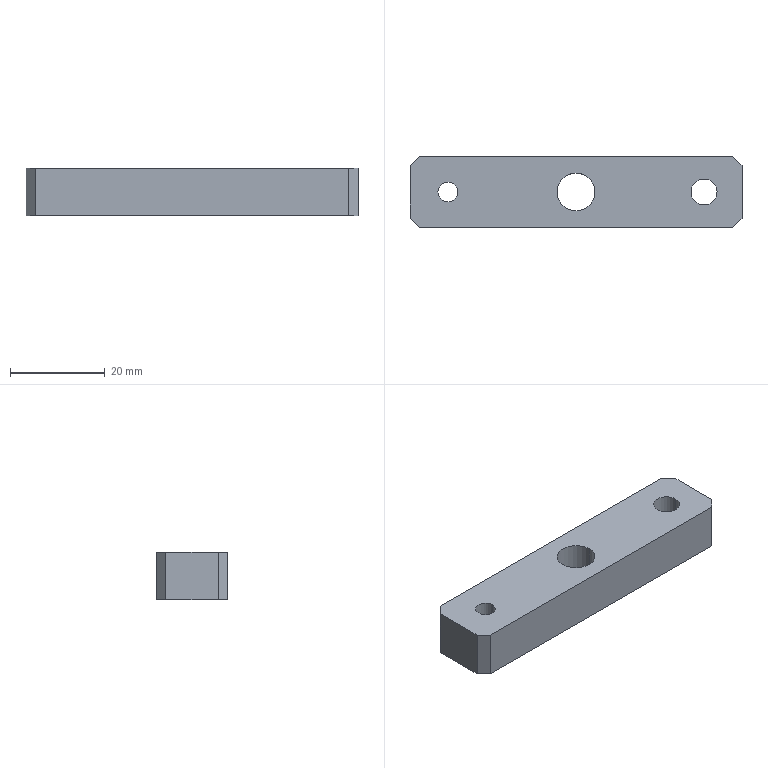Part | STEP file | 2015 Stopper | 1 solid | 19 faces | box 70 x 15 x 10 mm | volume 9229 mm3 | plane 11 | cylinder 8 | commonest cylinder face diameters 4.2 x2 5.5 x2 8 x2 10 x2
STEP:
#1=CARTESIAN_POINT('',(0.,0.,0.));
#2=DIRECTION('',(0.,0.,1.));
#3=DIRECTION('',(1.,0.,0.));
#4=AXIS2_PLACEMENT_3D('',#1,#2,#3);
#5=CARTESIAN_POINT('',(22.,0.,5.7));
#6=VERTEX_POINT('',#5);
#7=CARTESIAN_POINT('',(22.,0.,0.));
#8=VERTEX_POINT('',#7);
#9=CARTESIAN_POINT('',(22.,0.,0.));
#10=DIRECTION('',(0.,0.,-1.));
#11=VECTOR('',#10,1.);
#12=LINE('',#9,#11);
#13=CARTESIAN_POINT('',(27.,0.,0.));
#14=DIRECTION('',(0.,0.,-1.));
#15=DIRECTION('',(-1.,0.,0.));
#16=AXIS2_PLACEMENT_3D('',#13,#14,#15);
#17=CYLINDRICAL_SURFACE('',#16,5.);
#18=CARTESIAN_POINT('',(6.283,0.));
#19=DIRECTION('',(0.,1.));
#20=VECTOR('',#19,1.);
#21=LINE('',#18,#20);
#22=(GEOMETRIC_REPRESENTATION_CONTEXT(2)PARAMETRIC_REPRESENTATION_CONTEXT()REPRESENTATION_CONTEXT('',''));
#23=DEFINITIONAL_REPRESENTATION('',(#21),#22);
#24=PCURVE('',#17,#23);
#25=CARTESIAN_POINT('',(27.,0.,0.));
#26=DIRECTION('',(0.,0.,-1.));
#27=DIRECTION('',(-1.,0.,0.));
#28=AXIS2_PLACEMENT_3D('',#25,#26,#27);
#29=CYLINDRICAL_SURFACE('',#28,5.);
#30=CARTESIAN_POINT('',(0.,0.));
#31=DIRECTION('',(0.,1.));
#32=VECTOR('',#31,1.);
#33=LINE('',#30,#32);
#34=(GEOMETRIC_REPRESENTATION_CONTEXT(2)PARAMETRIC_REPRESENTATION_CONTEXT()REPRESENTATION_CONTEXT('',''));
#35=DEFINITIONAL_REPRESENTATION('',(#33),#34);
#36=PCURVE('',#29,#35);
#37=SURFACE_CURVE('',#12,(#24,#36),.PCURVE_S1.);
#38=EDGE_CURVE('',#6,#8,#37,.T.);
#39=ORIENTED_EDGE('',*,*,#38,.T.);
#40=CARTESIAN_POINT('',(32.,0.,0.));
#41=VERTEX_POINT('',#40);
#42=CARTESIAN_POINT('',(27.,0.,0.));
#43=DIRECTION('',(0.,0.,-1.));
#44=DIRECTION('',(-1.,0.,0.));
#45=AXIS2_PLACEMENT_3D('',#42,#43,#44);
#46=CIRCLE('',#45,5.);
#47=CARTESIAN_POINT('',(0.,0.));
#48=DIRECTION('',(1.,0.));
#49=VECTOR('',#48,1.);
#50=LINE('',#47,#49);
#51=(GEOMETRIC_REPRESENTATION_CONTEXT(2)PARAMETRIC_REPRESENTATION_CONTEXT()REPRESENTATION_CONTEXT('',''));
#52=DEFINITIONAL_REPRESENTATION('',(#50),#51);
#53=PCURVE('',#17,#52);
#54=CARTESIAN_POINT('',(0.,0.,0.));
#55=DIRECTION('',(0.,0.,-1.));
#56=DIRECTION('',(-1.,0.,0.));
#57=AXIS2_PLACEMENT_3D('',#54,#55,#56);
#58=PLANE('',#57);
#59=CARTESIAN_POINT('',(-27.,0.));
#60=DIRECTION('',(1.,0.));
#61=AXIS2_PLACEMENT_2D('',#59,#60);
#62=CIRCLE('',#61,5.);
#63=(GEOMETRIC_REPRESENTATION_CONTEXT(2)PARAMETRIC_REPRESENTATION_CONTEXT()REPRESENTATION_CONTEXT('',''));
#64=DEFINITIONAL_REPRESENTATION('',(#62),#63);
#65=PCURVE('',#58,#64);
#66=SURFACE_CURVE('',#46,(#53,#65),.PCURVE_S1.);
#67=EDGE_CURVE('',#41,#8,#66,.T.);
#68=ORIENTED_EDGE('',*,*,#67,.F.);
#69=CARTESIAN_POINT('',(32.,0.,5.7));
#70=VERTEX_POINT('',#69);
#71=CARTESIAN_POINT('',(32.,0.,0.));
#72=DIRECTION('',(0.,0.,-1.));
#73=VECTOR('',#72,1.);
#74=LINE('',#71,#73);
#75=CARTESIAN_POINT('',(3.142,0.));
#76=DIRECTION('',(0.,1.));
#77=VECTOR('',#76,1.);
#78=LINE('',#75,#77);
#79=(GEOMETRIC_REPRESENTATION_CONTEXT(2)PARAMETRIC_REPRESENTATION_CONTEXT()REPRESENTATION_CONTEXT('',''));
#80=DEFINITIONAL_REPRESENTATION('',(#78),#79);
#81=PCURVE('',#17,#80);
#82=CARTESIAN_POINT('',(3.142,0.));
#83=DIRECTION('',(0.,1.));
#84=VECTOR('',#83,1.);
#85=LINE('',#82,#84);
#86=(GEOMETRIC_REPRESENTATION_CONTEXT(2)PARAMETRIC_REPRESENTATION_CONTEXT()REPRESENTATION_CONTEXT('',''));
#87=DEFINITIONAL_REPRESENTATION('',(#85),#86);
#88=PCURVE('',#29,#87);
#89=SURFACE_CURVE('',#74,(#81,#88),.PCURVE_S1.);
#90=EDGE_CURVE('',#70,#41,#89,.T.);
#91=ORIENTED_EDGE('',*,*,#90,.F.);
#92=CARTESIAN_POINT('',(27.,0.,5.7));
#93=DIRECTION('',(0.,0.,-1.));
#94=DIRECTION('',(-1.,0.,0.));
#95=AXIS2_PLACEMENT_3D('',#92,#93,#94);
#96=CIRCLE('',#95,5.);
#97=CARTESIAN_POINT('',(0.,-5.7));
#98=DIRECTION('',(1.,0.));
#99=VECTOR('',#98,1.);
#100=LINE('',#97,#99);
#101=(GEOMETRIC_REPRESENTATION_CONTEXT(2)PARAMETRIC_REPRESENTATION_CONTEXT()REPRESENTATION_CONTEXT('',''));
#102=DEFINITIONAL_REPRESENTATION('',(#100),#101);
#103=PCURVE('',#17,#102);
#104=CARTESIAN_POINT('',(29.75,0.,5.7));
#105=DIRECTION('',(0.,0.,1.));
#106=DIRECTION('',(1.,0.,0.));
#107=AXIS2_PLACEMENT_3D('',#104,#105,#106);
#108=PLANE('',#107);
#109=CARTESIAN_POINT('',(-7.75,0.));
#110=CARTESIAN_POINT('',(-7.75,8.66));
#111=CARTESIAN_POINT('',(-0.25,4.33));
#112=CARTESIAN_POINT('',(7.25,0.));
#113=CARTESIAN_POINT('',(-0.25,-4.33));
#114=CARTESIAN_POINT('',(-7.75,-8.66));
#115=CARTESIAN_POINT('',(-7.75,0.));
#116=(BOUNDED_CURVE()B_SPLINE_CURVE(2,(#109,#110,#111,#112,#113,#114,#115),.UNSPECIFIED.,.T.,.F.)B_SPLINE_CURVE_WITH_KNOTS((1,2,2,2,2,1),(-2.094,0.,2.094,4.189,6.283,8.378),.UNSPECIFIED.)CURVE()GEOMETRIC_REPRESENTATION_ITEM()RATIONAL_B_SPLINE_CURVE((1.,0.5,1.,0.5,1.,0.5,1.))REPRESENTATION_ITEM(''));
#117=(GEOMETRIC_REPRESENTATION_CONTEXT(2)PARAMETRIC_REPRESENTATION_CONTEXT()REPRESENTATION_CONTEXT('',''));
#118=DEFINITIONAL_REPRESENTATION('',(#116),#117);
#119=PCURVE('',#108,#118);
#120=SURFACE_CURVE('',#96,(#103,#119),.PCURVE_S1.);
#121=EDGE_CURVE('',#70,#6,#120,.T.);
#122=ORIENTED_EDGE('',*,*,#121,.T.);
#123=EDGE_LOOP('',(#39,#68,#91,#122));
#124=FACE_BOUND('',#123,.F.);
#125=ADVANCED_FACE('',(#124),#17,.F.);
#126=CARTESIAN_POINT('',(24.25,0.,10.));
#127=VERTEX_POINT('',#126);
#128=CARTESIAN_POINT('',(24.25,0.,5.7));
#129=VERTEX_POINT('',#128);
#130=CARTESIAN_POINT('',(24.25,0.,0.));
#131=DIRECTION('',(0.,0.,-1.));
#132=VECTOR('',#131,1.);
#133=LINE('',#130,#132);
#134=CARTESIAN_POINT('',(27.,0.,0.));
#135=DIRECTION('',(0.,0.,-1.));
#136=DIRECTION('',(-1.,0.,0.));
#137=AXIS2_PLACEMENT_3D('',#134,#135,#136);
#138=CYLINDRICAL_SURFACE('',#137,2.75);
#139=CARTESIAN_POINT('',(6.283,0.));
#140=DIRECTION('',(0.,1.));
#141=VECTOR('',#140,1.);
#142=LINE('',#139,#141);
#143=(GEOMETRIC_REPRESENTATION_CONTEXT(2)PARAMETRIC_REPRESENTATION_CONTEXT()REPRESENTATION_CONTEXT('',''));
#144=DEFINITIONAL_REPRESENTATION('',(#142),#143);
#145=PCURVE('',#138,#144);
#146=CARTESIAN_POINT('',(27.,0.,0.));
#147=DIRECTION('',(0.,0.,-1.));
#148=DIRECTION('',(-1.,0.,0.));
#149=AXIS2_PLACEMENT_3D('',#146,#147,#148);
#150=CYLINDRICAL_SURFACE('',#149,2.75);
#151=CARTESIAN_POINT('',(0.,0.));
#152=DIRECTION('',(0.,1.));
#153=VECTOR('',#152,1.);
#154=LINE('',#151,#153);
#155=(GEOMETRIC_REPRESENTATION_CONTEXT(2)PARAMETRIC_REPRESENTATION_CONTEXT()REPRESENTATION_CONTEXT('',''));
#156=DEFINITIONAL_REPRESENTATION('',(#154),#155);
#157=PCURVE('',#150,#156);
#158=SURFACE_CURVE('',#133,(#145,#157),.PCURVE_S1.);
#159=EDGE_CURVE('',#127,#129,#158,.T.);
#160=ORIENTED_EDGE('',*,*,#159,.T.);
#161=CARTESIAN_POINT('',(29.75,0.,5.7));
#162=VERTEX_POINT('',#161);
#163=CARTESIAN_POINT('',(27.,0.,5.7));
#164=DIRECTION('',(0.,0.,-1.));
#165=DIRECTION('',(-1.,0.,0.));
#166=AXIS2_PLACEMENT_3D('',#163,#164,#165);
#167=CIRCLE('',#166,2.75);
#168=CARTESIAN_POINT('',(0.,-5.7));
#169=DIRECTION('',(1.,0.));
#170=VECTOR('',#169,1.);
#171=LINE('',#168,#170);
#172=(GEOMETRIC_REPRESENTATION_CONTEXT(2)PARAMETRIC_REPRESENTATION_CONTEXT()REPRESENTATION_CONTEXT('',''));
#173=DEFINITIONAL_REPRESENTATION('',(#171),#172);
#174=PCURVE('',#138,#173);
#175=CARTESIAN_POINT('',(-5.5,0.));
#176=CARTESIAN_POINT('',(-5.5,4.763));
#177=CARTESIAN_POINT('',(-1.375,2.382));
#178=CARTESIAN_POINT('',(2.75,0.));
#179=CARTESIAN_POINT('',(-1.375,-2.382));
#180=CARTESIAN_POINT('',(-5.5,-4.763));
#181=CARTESIAN_POINT('',(-5.5,0.));
#182=(BOUNDED_CURVE()B_SPLINE_CURVE(2,(#175,#176,#177,#178,#179,#180,#181),.UNSPECIFIED.,.T.,.F.)B_SPLINE_CURVE_WITH_KNOTS((1,2,2,2,2,1),(-2.094,0.,2.094,4.189,6.283,8.378),.UNSPECIFIED.)CURVE()GEOMETRIC_REPRESENTATION_ITEM()RATIONAL_B_SPLINE_CURVE((1.,0.5,1.,0.5,1.,0.5,1.))REPRESENTATION_ITEM(''));
#183=(GEOMETRIC_REPRESENTATION_CONTEXT(2)PARAMETRIC_REPRESENTATION_CONTEXT()REPRESENTATION_CONTEXT('',''));
#184=DEFINITIONAL_REPRESENTATION('',(#182),#183);
#185=PCURVE('',#108,#184);
#186=SURFACE_CURVE('',#167,(#174,#185),.PCURVE_S1.);
#187=EDGE_CURVE('',#162,#129,#186,.T.);
#188=ORIENTED_EDGE('',*,*,#187,.F.);
#189=CARTESIAN_POINT('',(29.75,0.,10.));
#190=VERTEX_POINT('',#189);
#191=CARTESIAN_POINT('',(29.75,0.,0.));
#192=DIRECTION('',(0.,0.,-1.));
#193=VECTOR('',#192,1.);
#194=LINE('',#191,#193);
#195=CARTESIAN_POINT('',(3.142,0.));
#196=DIRECTION('',(0.,1.));
#197=VECTOR('',#196,1.);
#198=LINE('',#195,#197);
#199=(GEOMETRIC_REPRESENTATION_CONTEXT(2)PARAMETRIC_REPRESENTATION_CONTEXT()REPRESENTATION_CONTEXT('',''));
#200=DEFINITIONAL_REPRESENTATION('',(#198),#199);
#201=PCURVE('',#138,#200);
#202=CARTESIAN_POINT('',(3.142,0.));
#203=DIRECTION('',(0.,1.));
#204=VECTOR('',#203,1.);
#205=LINE('',#202,#204);
#206=(GEOMETRIC_REPRESENTATION_CONTEXT(2)PARAMETRIC_REPRESENTATION_CONTEXT()REPRESENTATION_CONTEXT('',''));
#207=DEFINITIONAL_REPRESENTATION('',(#205),#206);
#208=PCURVE('',#150,#207);
#209=SURFACE_CURVE('',#194,(#201,#208),.PCURVE_S1.);
#210=EDGE_CURVE('',#190,#162,#209,.T.);
#211=ORIENTED_EDGE('',*,*,#210,.F.);
#212=CARTESIAN_POINT('',(27.,0.,10.));
#213=DIRECTION('',(0.,0.,-1.));
#214=DIRECTION('',(-1.,0.,0.));
#215=AXIS2_PLACEMENT_3D('',#212,#213,#214);
#216=CIRCLE('',#215,2.75);
#217=CARTESIAN_POINT('',(0.,-10.));
#218=DIRECTION('',(1.,0.));
#219=VECTOR('',#218,1.);
#220=LINE('',#217,#219);
#221=(GEOMETRIC_REPRESENTATION_CONTEXT(2)PARAMETRIC_REPRESENTATION_CONTEXT()REPRESENTATION_CONTEXT('',''));
#222=DEFINITIONAL_REPRESENTATION('',(#220),#221);
#223=PCURVE('',#138,#222);
#224=CARTESIAN_POINT('',(0.,0.,10.));
#225=DIRECTION('',(0.,0.,-1.));
#226=DIRECTION('',(-1.,0.,0.));
#227=AXIS2_PLACEMENT_3D('',#224,#225,#226);
#228=PLANE('',#227);
#229=CARTESIAN_POINT('',(-27.,0.));
#230=DIRECTION('',(1.,0.));
#231=AXIS2_PLACEMENT_2D('',#229,#230);
#232=CIRCLE('',#231,2.75);
#233=(GEOMETRIC_REPRESENTATION_CONTEXT(2)PARAMETRIC_REPRESENTATION_CONTEXT()REPRESENTATION_CONTEXT('',''));
#234=DEFINITIONAL_REPRESENTATION('',(#232),#233);
#235=PCURVE('',#228,#234);
#236=SURFACE_CURVE('',#216,(#223,#235),.PCURVE_S1.);
#237=EDGE_CURVE('',#190,#127,#236,.T.);
#238=ORIENTED_EDGE('',*,*,#237,.T.);
#239=EDGE_LOOP('',(#160,#188,#211,#238));
#240=FACE_BOUND('',#239,.F.);
#241=ADVANCED_FACE('',(#240),#138,.F.);
#242=CARTESIAN_POINT('',(-24.9,0.,0.));
#243=VERTEX_POINT('',#242);
#244=CARTESIAN_POINT('',(-24.9,0.,10.));
#245=VERTEX_POINT('',#244);
#246=CARTESIAN_POINT('',(-24.9,0.,10.));
#247=DIRECTION('',(0.,0.,1.));
#248=VECTOR('',#247,1.);
#249=LINE('',#246,#248);
#250=CARTESIAN_POINT('',(-27.,0.,10.));
#251=DIRECTION('',(0.,0.,1.));
#252=DIRECTION('',(1.,0.,0.));
#253=AXIS2_PLACEMENT_3D('',#250,#251,#252);
#254=CYLINDRICAL_SURFACE('',#253,2.1);
#255=CARTESIAN_POINT('',(6.283,0.));
#256=DIRECTION('',(0.,1.));
#257=VECTOR('',#256,1.);
#258=LINE('',#255,#257);
#259=(GEOMETRIC_REPRESENTATION_CONTEXT(2)PARAMETRIC_REPRESENTATION_CONTEXT()REPRESENTATION_CONTEXT('',''));
#260=DEFINITIONAL_REPRESENTATION('',(#258),#259);
#261=PCURVE('',#254,#260);
#262=CARTESIAN_POINT('',(-27.,0.,10.));
#263=DIRECTION('',(0.,0.,1.));
#264=DIRECTION('',(1.,0.,0.));
#265=AXIS2_PLACEMENT_3D('',#262,#263,#264);
#266=CYLINDRICAL_SURFACE('',#265,2.1);
#267=CARTESIAN_POINT('',(0.,0.));
#268=DIRECTION('',(0.,1.));
#269=VECTOR('',#268,1.);
#270=LINE('',#267,#269);
#271=(GEOMETRIC_REPRESENTATION_CONTEXT(2)PARAMETRIC_REPRESENTATION_CONTEXT()REPRESENTATION_CONTEXT('',''));
#272=DEFINITIONAL_REPRESENTATION('',(#270),#271);
#273=PCURVE('',#266,#272);
#274=SURFACE_CURVE('',#249,(#261,#273),.PCURVE_S1.);
#275=EDGE_CURVE('',#243,#245,#274,.T.);
#276=ORIENTED_EDGE('',*,*,#275,.T.);
#277=CARTESIAN_POINT('',(-29.1,0.,10.));
#278=VERTEX_POINT('',#277);
#279=CARTESIAN_POINT('',(-27.,0.,10.));
#280=DIRECTION('',(0.,0.,1.));
#281=DIRECTION('',(1.,0.,0.));
#282=AXIS2_PLACEMENT_3D('',#279,#280,#281);
#283=CIRCLE('',#282,2.1);
#284=CARTESIAN_POINT('',(0.,0.));
#285=DIRECTION('',(1.,0.));
#286=VECTOR('',#285,1.);
#287=LINE('',#284,#286);
#288=(GEOMETRIC_REPRESENTATION_CONTEXT(2)PARAMETRIC_REPRESENTATION_CONTEXT()REPRESENTATION_CONTEXT('',''));
#289=DEFINITIONAL_REPRESENTATION('',(#287),#288);
#290=PCURVE('',#254,#289);
#291=CARTESIAN_POINT('',(24.9,0.));
#292=CARTESIAN_POINT('',(24.9,3.637));
#293=CARTESIAN_POINT('',(28.05,1.819));
#294=CARTESIAN_POINT('',(31.2,0.));
#295=CARTESIAN_POINT('',(28.05,-1.819));
#296=CARTESIAN_POINT('',(24.9,-3.637));
#297=CARTESIAN_POINT('',(24.9,0.));
#298=(BOUNDED_CURVE()B_SPLINE_CURVE(2,(#291,#292,#293,#294,#295,#296,#297),.UNSPECIFIED.,.T.,.F.)B_SPLINE_CURVE_WITH_KNOTS((1,2,2,2,2,1),(-2.094,0.,2.094,4.189,6.283,8.378),.UNSPECIFIED.)CURVE()GEOMETRIC_REPRESENTATION_ITEM()RATIONAL_B_SPLINE_CURVE((1.,0.5,1.,0.5,1.,0.5,1.))REPRESENTATION_ITEM(''));
#299=(GEOMETRIC_REPRESENTATION_CONTEXT(2)PARAMETRIC_REPRESENTATION_CONTEXT()REPRESENTATION_CONTEXT('',''));
#300=DEFINITIONAL_REPRESENTATION('',(#298),#299);
#301=PCURVE('',#228,#300);
#302=SURFACE_CURVE('',#283,(#290,#301),.PCURVE_S1.);
#303=EDGE_CURVE('',#278,#245,#302,.T.);
#304=ORIENTED_EDGE('',*,*,#303,.F.);
#305=CARTESIAN_POINT('',(-29.1,0.,0.));
#306=VERTEX_POINT('',#305);
#307=CARTESIAN_POINT('',(-29.1,0.,10.));
#308=DIRECTION('',(0.,0.,1.));
#309=VECTOR('',#308,1.);
#310=LINE('',#307,#309);
#311=CARTESIAN_POINT('',(3.142,0.));
#312=DIRECTION('',(0.,1.));
#313=VECTOR('',#312,1.);
#314=LINE('',#311,#313);
#315=(GEOMETRIC_REPRESENTATION_CONTEXT(2)PARAMETRIC_REPRESENTATION_CONTEXT()REPRESENTATION_CONTEXT('',''));
#316=DEFINITIONAL_REPRESENTATION('',(#314),#315);
#317=PCURVE('',#254,#316);
#318=CARTESIAN_POINT('',(3.142,0.));
#319=DIRECTION('',(0.,1.));
#320=VECTOR('',#319,1.);
#321=LINE('',#318,#320);
#322=(GEOMETRIC_REPRESENTATION_CONTEXT(2)PARAMETRIC_REPRESENTATION_CONTEXT()REPRESENTATION_CONTEXT('',''));
#323=DEFINITIONAL_REPRESENTATION('',(#321),#322);
#324=PCURVE('',#266,#323);
#325=SURFACE_CURVE('',#310,(#317,#324),.PCURVE_S1.);
#326=EDGE_CURVE('',#306,#278,#325,.T.);
#327=ORIENTED_EDGE('',*,*,#326,.F.);
#328=CARTESIAN_POINT('',(-27.,0.,0.));
#329=DIRECTION('',(0.,0.,-1.));
#330=DIRECTION('',(-1.,0.,0.));
#331=AXIS2_PLACEMENT_3D('',#328,#329,#330);
#332=CIRCLE('',#331,2.1);
#333=CARTESIAN_POINT('',(9.425,-10.));
#334=DIRECTION('',(-1.,0.));
#335=VECTOR('',#334,1.);
#336=LINE('',#333,#335);
#337=(GEOMETRIC_REPRESENTATION_CONTEXT(2)PARAMETRIC_REPRESENTATION_CONTEXT()REPRESENTATION_CONTEXT('',''));
#338=DEFINITIONAL_REPRESENTATION('',(#336),#337);
#339=PCURVE('',#254,#338);
#340=CARTESIAN_POINT('',(27.,0.));
#341=DIRECTION('',(1.,0.));
#342=AXIS2_PLACEMENT_2D('',#340,#341);
#343=CIRCLE('',#342,2.1);
#344=(GEOMETRIC_REPRESENTATION_CONTEXT(2)PARAMETRIC_REPRESENTATION_CONTEXT()REPRESENTATION_CONTEXT('',''));
#345=DEFINITIONAL_REPRESENTATION('',(#343),#344);
#346=PCURVE('',#58,#345);
#347=SURFACE_CURVE('',#332,(#339,#346),.PCURVE_S1.);
#348=EDGE_CURVE('',#243,#306,#347,.T.);
#349=ORIENTED_EDGE('',*,*,#348,.F.);
#350=EDGE_LOOP('',(#276,#304,#327,#349));
#351=FACE_BOUND('',#350,.F.);
#352=ADVANCED_FACE('',(#351),#254,.F.);
#353=CARTESIAN_POINT('',(4.,0.,0.));
#354=VERTEX_POINT('',#353);
#355=CARTESIAN_POINT('',(4.,0.,10.));
#356=VERTEX_POINT('',#355);
#357=CARTESIAN_POINT('',(4.,0.,0.));
#358=DIRECTION('',(0.,0.,1.));
#359=VECTOR('',#358,1.);
#360=LINE('',#357,#359);
#361=CARTESIAN_POINT('',(0.,0.,0.));
#362=DIRECTION('',(0.,0.,1.));
#363=DIRECTION('',(1.,0.,0.));
#364=AXIS2_PLACEMENT_3D('',#361,#362,#363);
#365=CYLINDRICAL_SURFACE('',#364,4.);
#366=CARTESIAN_POINT('',(6.283,0.));
#367=DIRECTION('',(0.,1.));
#368=VECTOR('',#367,1.);
#369=LINE('',#366,#368);
#370=(GEOMETRIC_REPRESENTATION_CONTEXT(2)PARAMETRIC_REPRESENTATION_CONTEXT()REPRESENTATION_CONTEXT('',''));
#371=DEFINITIONAL_REPRESENTATION('',(#369),#370);
#372=PCURVE('',#365,#371);
#373=CARTESIAN_POINT('',(0.,0.,0.));
#374=DIRECTION('',(0.,0.,1.));
#375=DIRECTION('',(1.,0.,0.));
#376=AXIS2_PLACEMENT_3D('',#373,#374,#375);
#377=CYLINDRICAL_SURFACE('',#376,4.);
#378=CARTESIAN_POINT('',(0.,0.));
#379=DIRECTION('',(0.,1.));
#380=VECTOR('',#379,1.);
#381=LINE('',#378,#380);
#382=(GEOMETRIC_REPRESENTATION_CONTEXT(2)PARAMETRIC_REPRESENTATION_CONTEXT()REPRESENTATION_CONTEXT('',''));
#383=DEFINITIONAL_REPRESENTATION('',(#381),#382);
#384=PCURVE('',#377,#383);
#385=SURFACE_CURVE('',#360,(#372,#384),.PCURVE_S1.);
#386=EDGE_CURVE('',#354,#356,#385,.T.);
#387=ORIENTED_EDGE('',*,*,#386,.T.);
#388=CARTESIAN_POINT('',(-4.,0.,10.));
#389=VERTEX_POINT('',#388);
#390=CARTESIAN_POINT('',(0.,0.,10.));
#391=DIRECTION('',(0.,0.,1.));
#392=DIRECTION('',(1.,0.,0.));
#393=AXIS2_PLACEMENT_3D('',#390,#391,#392);
#394=CIRCLE('',#393,4.);
#395=CARTESIAN_POINT('',(0.,10.));
#396=DIRECTION('',(1.,0.));
#397=VECTOR('',#396,1.);
#398=LINE('',#395,#397);
#399=(GEOMETRIC_REPRESENTATION_CONTEXT(2)PARAMETRIC_REPRESENTATION_CONTEXT()REPRESENTATION_CONTEXT('',''));
#400=DEFINITIONAL_REPRESENTATION('',(#398),#399);
#401=PCURVE('',#365,#400);
#402=CARTESIAN_POINT('',(-4.,0.));
#403=CARTESIAN_POINT('',(-4.,6.928));
#404=CARTESIAN_POINT('',(2.,3.464));
#405=CARTESIAN_POINT('',(8.,0.));
#406=CARTESIAN_POINT('',(2.,-3.464));
#407=CARTESIAN_POINT('',(-4.,-6.928));
#408=CARTESIAN_POINT('',(-4.,0.));
#409=(BOUNDED_CURVE()B_SPLINE_CURVE(2,(#402,#403,#404,#405,#406,#407,#408),.UNSPECIFIED.,.T.,.F.)B_SPLINE_CURVE_WITH_KNOTS((1,2,2,2,2,1),(-2.094,0.,2.094,4.189,6.283,8.378),.UNSPECIFIED.)CURVE()GEOMETRIC_REPRESENTATION_ITEM()RATIONAL_B_SPLINE_CURVE((1.,0.5,1.,0.5,1.,0.5,1.))REPRESENTATION_ITEM(''));
#410=(GEOMETRIC_REPRESENTATION_CONTEXT(2)PARAMETRIC_REPRESENTATION_CONTEXT()REPRESENTATION_CONTEXT('',''));
#411=DEFINITIONAL_REPRESENTATION('',(#409),#410);
#412=PCURVE('',#228,#411);
#413=SURFACE_CURVE('',#394,(#401,#412),.PCURVE_S1.);
#414=EDGE_CURVE('',#389,#356,#413,.T.);
#415=ORIENTED_EDGE('',*,*,#414,.F.);
#416=CARTESIAN_POINT('',(-4.,0.,0.));
#417=VERTEX_POINT('',#416);
#418=CARTESIAN_POINT('',(-4.,0.,0.));
#419=DIRECTION('',(0.,0.,1.));
#420=VECTOR('',#419,1.);
#421=LINE('',#418,#420);
#422=CARTESIAN_POINT('',(3.142,0.));
#423=DIRECTION('',(0.,1.));
#424=VECTOR('',#423,1.);
#425=LINE('',#422,#424);
#426=(GEOMETRIC_REPRESENTATION_CONTEXT(2)PARAMETRIC_REPRESENTATION_CONTEXT()REPRESENTATION_CONTEXT('',''));
#427=DEFINITIONAL_REPRESENTATION('',(#425),#426);
#428=PCURVE('',#365,#427);
#429=CARTESIAN_POINT('',(3.142,0.));
#430=DIRECTION('',(0.,1.));
#431=VECTOR('',#430,1.);
#432=LINE('',#429,#431);
#433=(GEOMETRIC_REPRESENTATION_CONTEXT(2)PARAMETRIC_REPRESENTATION_CONTEXT()REPRESENTATION_CONTEXT('',''));
#434=DEFINITIONAL_REPRESENTATION('',(#432),#433);
#435=PCURVE('',#377,#434);
#436=SURFACE_CURVE('',#421,(#428,#435),.PCURVE_S1.);
#437=EDGE_CURVE('',#417,#389,#436,.T.);
#438=ORIENTED_EDGE('',*,*,#437,.F.);
#439=CARTESIAN_POINT('',(0.,0.,0.));
#440=DIRECTION('',(0.,0.,1.));
#441=DIRECTION('',(1.,0.,0.));
#442=AXIS2_PLACEMENT_3D('',#439,#440,#441);
#443=CIRCLE('',#442,4.);
#444=CARTESIAN_POINT('',(0.,0.));
#445=DIRECTION('',(1.,0.));
#446=VECTOR('',#445,1.);
#447=LINE('',#444,#446);
#448=(GEOMETRIC_REPRESENTATION_CONTEXT(2)PARAMETRIC_REPRESENTATION_CONTEXT()REPRESENTATION_CONTEXT('',''));
#449=DEFINITIONAL_REPRESENTATION('',(#447),#448);
#450=PCURVE('',#365,#449);
#451=CARTESIAN_POINT('',(-4.,0.));
#452=CARTESIAN_POINT('',(-4.,6.928));
#453=CARTESIAN_POINT('',(2.,3.464));
#454=CARTESIAN_POINT('',(8.,0.));
#455=CARTESIAN_POINT('',(2.,-3.464));
#456=CARTESIAN_POINT('',(-4.,-6.928));
#457=CARTESIAN_POINT('',(-4.,0.));
#458=(BOUNDED_CURVE()B_SPLINE_CURVE(2,(#451,#452,#453,#454,#455,#456,#457),.UNSPECIFIED.,.T.,.F.)B_SPLINE_CURVE_WITH_KNOTS((1,2,2,2,2,1),(-2.094,0.,2.094,4.189,6.283,8.378),.UNSPECIFIED.)CURVE()GEOMETRIC_REPRESENTATION_ITEM()RATIONAL_B_SPLINE_CURVE((1.,0.5,1.,0.5,1.,0.5,1.))REPRESENTATION_ITEM(''));
#459=(GEOMETRIC_REPRESENTATION_CONTEXT(2)PARAMETRIC_REPRESENTATION_CONTEXT()REPRESENTATION_CONTEXT('',''));
#460=DEFINITIONAL_REPRESENTATION('',(#458),#459);
#461=PCURVE('',#58,#460);
#462=SURFACE_CURVE('',#443,(#450,#461),.PCURVE_S1.);
#463=EDGE_CURVE('',#417,#354,#462,.T.);
#464=ORIENTED_EDGE('',*,*,#463,.T.);
#465=EDGE_LOOP('',(#387,#415,#438,#464));
#466=FACE_BOUND('',#465,.F.);
#467=ADVANCED_FACE('',(#466),#365,.F.);
#468=CARTESIAN_POINT('',(27.,0.,10.));
#469=DIRECTION('',(0.,0.,-1.));
#470=DIRECTION('',(-1.,0.,0.));
#471=AXIS2_PLACEMENT_3D('',#468,#469,#470);
#472=CIRCLE('',#471,2.75);
#473=CARTESIAN_POINT('',(-27.,0.));
#474=DIRECTION('',(1.,0.));
#475=AXIS2_PLACEMENT_2D('',#473,#474);
#476=CIRCLE('',#475,2.75);
#477=(GEOMETRIC_REPRESENTATION_CONTEXT(2)PARAMETRIC_REPRESENTATION_CONTEXT()REPRESENTATION_CONTEXT('',''));
#478=DEFINITIONAL_REPRESENTATION('',(#476),#477);
#479=PCURVE('',#228,#478);
#480=CARTESIAN_POINT('',(0.,-10.));
#481=DIRECTION('',(1.,0.));
#482=VECTOR('',#481,1.);
#483=LINE('',#480,#482);
#484=(GEOMETRIC_REPRESENTATION_CONTEXT(2)PARAMETRIC_REPRESENTATION_CONTEXT()REPRESENTATION_CONTEXT('',''));
#485=DEFINITIONAL_REPRESENTATION('',(#483),#484);
#486=PCURVE('',#150,#485);
#487=SURFACE_CURVE('',#472,(#479,#486),.PCURVE_S1.);
#488=EDGE_CURVE('',#127,#190,#487,.T.);
#489=ORIENTED_EDGE('',*,*,#488,.T.);
#490=ORIENTED_EDGE('',*,*,#237,.T.);
#491=EDGE_LOOP('',(#489,#490));
#492=FACE_BOUND('',#491,.T.);
#493=CARTESIAN_POINT('',(-35.,5.5,10.));
#494=VERTEX_POINT('',#493);
#495=CARTESIAN_POINT('',(-35.,-5.5,10.));
#496=VERTEX_POINT('',#495);
#497=CARTESIAN_POINT('',(-35.,-7.5,10.));
#498=DIRECTION('',(0.,-1.,0.));
#499=VECTOR('',#498,1.);
#500=LINE('',#497,#499);
#501=CARTESIAN_POINT('',(35.,-7.5));
#502=DIRECTION('',(0.,-1.));
#503=VECTOR('',#502,1.);
#504=LINE('',#501,#503);
#505=(GEOMETRIC_REPRESENTATION_CONTEXT(2)PARAMETRIC_REPRESENTATION_CONTEXT()REPRESENTATION_CONTEXT('',''));
#506=DEFINITIONAL_REPRESENTATION('',(#504),#505);
#507=PCURVE('',#228,#506);
#508=CARTESIAN_POINT('',(-35.,-7.5,10.));
#509=DIRECTION('',(1.,0.,0.));
#510=DIRECTION('',(0.,0.,-1.));
#511=AXIS2_PLACEMENT_3D('',#508,#509,#510);
#512=PLANE('',#511);
#513=CARTESIAN_POINT('',(0.,0.));
#514=DIRECTION('',(0.,-1.));
#515=VECTOR('',#514,1.);
#516=LINE('',#513,#515);
#517=(GEOMETRIC_REPRESENTATION_CONTEXT(2)PARAMETRIC_REPRESENTATION_CONTEXT()REPRESENTATION_CONTEXT('',''));
#518=DEFINITIONAL_REPRESENTATION('',(#516),#517);
#519=PCURVE('',#512,#518);
#520=SURFACE_CURVE('',#500,(#507,#519),.PCURVE_S1.);
#521=EDGE_CURVE('',#494,#496,#520,.T.);
#522=ORIENTED_EDGE('',*,*,#521,.T.);
#523=CARTESIAN_POINT('',(-33.,-7.5,10.));
#524=VERTEX_POINT('',#523);
#525=CARTESIAN_POINT('',(-33.,-7.5,10.));
#526=DIRECTION('',(0.7071,-0.7071,0.));
#527=VECTOR('',#526,1.);
#528=LINE('',#525,#527);
#529=CARTESIAN_POINT('',(33.,-7.5));
#530=DIRECTION('',(-0.7071,-0.7071));
#531=VECTOR('',#530,1.);
#532=LINE('',#529,#531);
#533=(GEOMETRIC_REPRESENTATION_CONTEXT(2)PARAMETRIC_REPRESENTATION_CONTEXT()REPRESENTATION_CONTEXT('',''));
#534=DEFINITIONAL_REPRESENTATION('',(#532),#533);
#535=PCURVE('',#228,#534);
#536=CARTESIAN_POINT('',(-33.,-7.5,10.));
#537=DIRECTION('',(0.7071,0.7071,0.));
#538=DIRECTION('',(0.,0.,-1.));
#539=AXIS2_PLACEMENT_3D('',#536,#537,#538);
#540=PLANE('',#539);
#541=CARTESIAN_POINT('',(0.,0.));
#542=DIRECTION('',(0.,-1.));
#543=VECTOR('',#542,1.);
#544=LINE('',#541,#543);
#545=(GEOMETRIC_REPRESENTATION_CONTEXT(2)PARAMETRIC_REPRESENTATION_CONTEXT()REPRESENTATION_CONTEXT('',''));
#546=DEFINITIONAL_REPRESENTATION('',(#544),#545);
#547=PCURVE('',#540,#546);
#548=SURFACE_CURVE('',#528,(#535,#547),.PCURVE_S1.);
#549=EDGE_CURVE('',#496,#524,#548,.T.);
#550=ORIENTED_EDGE('',*,*,#549,.T.);
#551=CARTESIAN_POINT('',(33.,-7.5,10.));
#552=VERTEX_POINT('',#551);
#553=CARTESIAN_POINT('',(-35.,-7.5,10.));
#554=DIRECTION('',(1.,0.,0.));
#555=VECTOR('',#554,1.);
#556=LINE('',#553,#555);
#557=CARTESIAN_POINT('',(35.,-7.5));
#558=DIRECTION('',(-1.,0.));
#559=VECTOR('',#558,1.);
#560=LINE('',#557,#559);
#561=(GEOMETRIC_REPRESENTATION_CONTEXT(2)PARAMETRIC_REPRESENTATION_CONTEXT()REPRESENTATION_CONTEXT('',''));
#562=DEFINITIONAL_REPRESENTATION('',(#560),#561);
#563=PCURVE('',#228,#562);
#564=CARTESIAN_POINT('',(-35.,-7.5,10.));
#565=DIRECTION('',(0.,1.,0.));
#566=DIRECTION('',(0.,0.,1.));
#567=AXIS2_PLACEMENT_3D('',#564,#565,#566);
#568=PLANE('',#567);
#569=CARTESIAN_POINT('',(0.,0.));
#570=DIRECTION('',(0.,1.));
#571=VECTOR('',#570,1.);
#572=LINE('',#569,#571);
#573=(GEOMETRIC_REPRESENTATION_CONTEXT(2)PARAMETRIC_REPRESENTATION_CONTEXT()REPRESENTATION_CONTEXT('',''));
#574=DEFINITIONAL_REPRESENTATION('',(#572),#573);
#575=PCURVE('',#568,#574);
#576=SURFACE_CURVE('',#556,(#563,#575),.PCURVE_S1.);
#577=EDGE_CURVE('',#524,#552,#576,.T.);
#578=ORIENTED_EDGE('',*,*,#577,.T.);
#579=CARTESIAN_POINT('',(35.,-5.5,10.));
#580=VERTEX_POINT('',#579);
#581=CARTESIAN_POINT('',(35.,-5.5,10.));
#582=DIRECTION('',(0.7071,0.7071,0.));
#583=VECTOR('',#582,1.);
#584=LINE('',#581,#583);
#585=CARTESIAN_POINT('',(-35.,-5.5));
#586=DIRECTION('',(-0.7071,0.7071));
#587=VECTOR('',#586,1.);
#588=LINE('',#585,#587);
#589=(GEOMETRIC_REPRESENTATION_CONTEXT(2)PARAMETRIC_REPRESENTATION_CONTEXT()REPRESENTATION_CONTEXT('',''));
#590=DEFINITIONAL_REPRESENTATION('',(#588),#589);
#591=PCURVE('',#228,#590);
#592=CARTESIAN_POINT('',(35.,-5.5,10.));
#593=DIRECTION('',(-0.7071,0.7071,0.));
#594=DIRECTION('',(0.,0.,-1.));
#595=AXIS2_PLACEMENT_3D('',#592,#593,#594);
#596=PLANE('',#595);
#597=CARTESIAN_POINT('',(0.,0.));
#598=DIRECTION('',(0.,-1.));
#599=VECTOR('',#598,1.);
#600=LINE('',#597,#599);
#601=(GEOMETRIC_REPRESENTATION_CONTEXT(2)PARAMETRIC_REPRESENTATION_CONTEXT()REPRESENTATION_CONTEXT('',''));
#602=DEFINITIONAL_REPRESENTATION('',(#600),#601);
#603=PCURVE('',#596,#602);
#604=SURFACE_CURVE('',#584,(#591,#603),.PCURVE_S1.);
#605=EDGE_CURVE('',#552,#580,#604,.T.);
#606=ORIENTED_EDGE('',*,*,#605,.T.);
#607=CARTESIAN_POINT('',(35.,5.5,10.));
#608=VERTEX_POINT('',#607);
#609=CARTESIAN_POINT('',(35.,-7.5,10.));
#610=DIRECTION('',(0.,1.,0.));
#611=VECTOR('',#610,1.);
#612=LINE('',#609,#611);
#613=CARTESIAN_POINT('',(-35.,-7.5));
#614=DIRECTION('',(0.,1.));
#615=VECTOR('',#614,1.);
#616=LINE('',#613,#615);
#617=(GEOMETRIC_REPRESENTATION_CONTEXT(2)PARAMETRIC_REPRESENTATION_CONTEXT()REPRESENTATION_CONTEXT('',''));
#618=DEFINITIONAL_REPRESENTATION('',(#616),#617);
#619=PCURVE('',#228,#618);
#620=CARTESIAN_POINT('',(35.,-7.5,10.));
#621=DIRECTION('',(-1.,0.,0.));
#622=DIRECTION('',(0.,0.,1.));
#623=AXIS2_PLACEMENT_3D('',#620,#621,#622);
#624=PLANE('',#623);
#625=CARTESIAN_POINT('',(0.,0.));
#626=DIRECTION('',(0.,1.));
#627=VECTOR('',#626,1.);
#628=LINE('',#625,#627);
#629=(GEOMETRIC_REPRESENTATION_CONTEXT(2)PARAMETRIC_REPRESENTATION_CONTEXT()REPRESENTATION_CONTEXT('',''));
#630=DEFINITIONAL_REPRESENTATION('',(#628),#629);
#631=PCURVE('',#624,#630);
#632=SURFACE_CURVE('',#612,(#619,#631),.PCURVE_S1.);
#633=EDGE_CURVE('',#580,#608,#632,.T.);
#634=ORIENTED_EDGE('',*,*,#633,.T.);
#635=CARTESIAN_POINT('',(33.,7.5,10.));
#636=VERTEX_POINT('',#635);
#637=CARTESIAN_POINT('',(33.,7.5,10.));
#638=DIRECTION('',(-0.7071,0.7071,0.));
#639=VECTOR('',#638,1.);
#640=LINE('',#637,#639);
#641=CARTESIAN_POINT('',(-33.,7.5));
#642=DIRECTION('',(0.7071,0.7071));
#643=VECTOR('',#642,1.);
#644=LINE('',#641,#643);
#645=(GEOMETRIC_REPRESENTATION_CONTEXT(2)PARAMETRIC_REPRESENTATION_CONTEXT()REPRESENTATION_CONTEXT('',''));
#646=DEFINITIONAL_REPRESENTATION('',(#644),#645);
#647=PCURVE('',#228,#646);
#648=CARTESIAN_POINT('',(33.,7.5,10.));
#649=DIRECTION('',(-0.7071,-0.7071,0.));
#650=DIRECTION('',(0.,0.,-1.));
#651=AXIS2_PLACEMENT_3D('',#648,#649,#650);
#652=PLANE('',#651);
#653=CARTESIAN_POINT('',(0.,0.));
#654=DIRECTION('',(0.,-1.));
#655=VECTOR('',#654,1.);
#656=LINE('',#653,#655);
#657=(GEOMETRIC_REPRESENTATION_CONTEXT(2)PARAMETRIC_REPRESENTATION_CONTEXT()REPRESENTATION_CONTEXT('',''));
#658=DEFINITIONAL_REPRESENTATION('',(#656),#657);
#659=PCURVE('',#652,#658);
#660=SURFACE_CURVE('',#640,(#647,#659),.PCURVE_S1.);
#661=EDGE_CURVE('',#608,#636,#660,.T.);
#662=ORIENTED_EDGE('',*,*,#661,.T.);
#663=CARTESIAN_POINT('',(-33.,7.5,10.));
#664=VERTEX_POINT('',#663);
#665=CARTESIAN_POINT('',(-35.,7.5,10.));
#666=DIRECTION('',(-1.,0.,0.));
#667=VECTOR('',#666,1.);
#668=LINE('',#665,#667);
#669=CARTESIAN_POINT('',(35.,7.5));
#670=DIRECTION('',(1.,0.));
#671=VECTOR('',#670,1.);
#672=LINE('',#669,#671);
#673=(GEOMETRIC_REPRESENTATION_CONTEXT(2)PARAMETRIC_REPRESENTATION_CONTEXT()REPRESENTATION_CONTEXT('',''));
#674=DEFINITIONAL_REPRESENTATION('',(#672),#673);
#675=PCURVE('',#228,#674);
#676=CARTESIAN_POINT('',(-35.,7.5,10.));
#677=DIRECTION('',(0.,-1.,0.));
#678=DIRECTION('',(0.,0.,-1.));
#679=AXIS2_PLACEMENT_3D('',#676,#677,#678);
#680=PLANE('',#679);
#681=CARTESIAN_POINT('',(0.,0.));
#682=DIRECTION('',(0.,-1.));
#683=VECTOR('',#682,1.);
#684=LINE('',#681,#683);
#685=(GEOMETRIC_REPRESENTATION_CONTEXT(2)PARAMETRIC_REPRESENTATION_CONTEXT()REPRESENTATION_CONTEXT('',''));
#686=DEFINITIONAL_REPRESENTATION('',(#684),#685);
#687=PCURVE('',#680,#686);
#688=SURFACE_CURVE('',#668,(#675,#687),.PCURVE_S1.);
#689=EDGE_CURVE('',#636,#664,#688,.T.);
#690=ORIENTED_EDGE('',*,*,#689,.T.);
#691=CARTESIAN_POINT('',(-35.,5.5,10.));
#692=DIRECTION('',(-0.7071,-0.7071,0.));
#693=VECTOR('',#692,1.);
#694=LINE('',#691,#693);
#695=CARTESIAN_POINT('',(35.,5.5));
#696=DIRECTION('',(0.7071,-0.7071));
#697=VECTOR('',#696,1.);
#698=LINE('',#695,#697);
#699=(GEOMETRIC_REPRESENTATION_CONTEXT(2)PARAMETRIC_REPRESENTATION_CONTEXT()REPRESENTATION_CONTEXT('',''));
#700=DEFINITIONAL_REPRESENTATION('',(#698),#699);
#701=PCURVE('',#228,#700);
#702=CARTESIAN_POINT('',(-35.,5.5,10.));
#703=DIRECTION('',(0.7071,-0.7071,0.));
#704=DIRECTION('',(0.,0.,-1.));
#705=AXIS2_PLACEMENT_3D('',#702,#703,#704);
#706=PLANE('',#705);
#707=CARTESIAN_POINT('',(0.,0.));
#708=DIRECTION('',(0.,-1.));
#709=VECTOR('',#708,1.);
#710=LINE('',#707,#709);
#711=(GEOMETRIC_REPRESENTATION_CONTEXT(2)PARAMETRIC_REPRESENTATION_CONTEXT()REPRESENTATION_CONTEXT('',''));
#712=DEFINITIONAL_REPRESENTATION('',(#710),#711);
#713=PCURVE('',#706,#712);
#714=SURFACE_CURVE('',#694,(#701,#713),.PCURVE_S1.);
#715=EDGE_CURVE('',#664,#494,#714,.T.);
#716=ORIENTED_EDGE('',*,*,#715,.T.);
#717=EDGE_LOOP('',(#522,#550,#578,#606,#634,#662,#690,#716));
#718=FACE_BOUND('',#717,.T.);
#719=CARTESIAN_POINT('',(0.,0.,10.));
#720=DIRECTION('',(0.,0.,1.));
#721=DIRECTION('',(1.,0.,0.));
#722=AXIS2_PLACEMENT_3D('',#719,#720,#721);
#723=CIRCLE('',#722,4.);
#724=CARTESIAN_POINT('',(-4.,0.));
#725=CARTESIAN_POINT('',(-4.,6.928));
#726=CARTESIAN_POINT('',(2.,3.464));
#727=CARTESIAN_POINT('',(8.,0.));
#728=CARTESIAN_POINT('',(2.,-3.464));
#729=CARTESIAN_POINT('',(-4.,-6.928));
#730=CARTESIAN_POINT('',(-4.,0.));
#731=(BOUNDED_CURVE()B_SPLINE_CURVE(2,(#724,#725,#726,#727,#728,#729,#730),.UNSPECIFIED.,.T.,.F.)B_SPLINE_CURVE_WITH_KNOTS((1,2,2,2,2,1),(-2.094,0.,2.094,4.189,6.283,8.378),.UNSPECIFIED.)CURVE()GEOMETRIC_REPRESENTATION_ITEM()RATIONAL_B_SPLINE_CURVE((1.,0.5,1.,0.5,1.,0.5,1.))REPRESENTATION_ITEM(''));
#732=(GEOMETRIC_REPRESENTATION_CONTEXT(2)PARAMETRIC_REPRESENTATION_CONTEXT()REPRESENTATION_CONTEXT('',''));
#733=DEFINITIONAL_REPRESENTATION('',(#731),#732);
#734=PCURVE('',#228,#733);
#735=CARTESIAN_POINT('',(0.,10.));
#736=DIRECTION('',(1.,0.));
#737=VECTOR('',#736,1.);
#738=LINE('',#735,#737);
#739=(GEOMETRIC_REPRESENTATION_CONTEXT(2)PARAMETRIC_REPRESENTATION_CONTEXT()REPRESENTATION_CONTEXT('',''));
#740=DEFINITIONAL_REPRESENTATION('',(#738),#739);
#741=PCURVE('',#377,#740);
#742=SURFACE_CURVE('',#723,(#734,#741),.PCURVE_S1.);
#743=EDGE_CURVE('',#356,#389,#742,.T.);
#744=ORIENTED_EDGE('',*,*,#743,.F.);
#745=ORIENTED_EDGE('',*,*,#414,.F.);
#746=EDGE_LOOP('',(#744,#745));
#747=FACE_BOUND('',#746,.T.);
#748=CARTESIAN_POINT('',(-27.,0.,10.));
#749=DIRECTION('',(0.,0.,1.));
#750=DIRECTION('',(1.,0.,0.));
#751=AXIS2_PLACEMENT_3D('',#748,#749,#750);
#752=CIRCLE('',#751,2.1);
#753=CARTESIAN_POINT('',(24.9,0.));
#754=CARTESIAN_POINT('',(24.9,3.637));
#755=CARTESIAN_POINT('',(28.05,1.819));
#756=CARTESIAN_POINT('',(31.2,0.));
#757=CARTESIAN_POINT('',(28.05,-1.819));
#758=CARTESIAN_POINT('',(24.9,-3.637));
#759=CARTESIAN_POINT('',(24.9,0.));
#760=(BOUNDED_CURVE()B_SPLINE_CURVE(2,(#753,#754,#755,#756,#757,#758,#759),.UNSPECIFIED.,.T.,.F.)B_SPLINE_CURVE_WITH_KNOTS((1,2,2,2,2,1),(-2.094,0.,2.094,4.189,6.283,8.378),.UNSPECIFIED.)CURVE()GEOMETRIC_REPRESENTATION_ITEM()RATIONAL_B_SPLINE_CURVE((1.,0.5,1.,0.5,1.,0.5,1.))REPRESENTATION_ITEM(''));
#761=(GEOMETRIC_REPRESENTATION_CONTEXT(2)PARAMETRIC_REPRESENTATION_CONTEXT()REPRESENTATION_CONTEXT('',''));
#762=DEFINITIONAL_REPRESENTATION('',(#760),#761);
#763=PCURVE('',#228,#762);
#764=CARTESIAN_POINT('',(0.,0.));
#765=DIRECTION('',(1.,0.));
#766=VECTOR('',#765,1.);
#767=LINE('',#764,#766);
#768=(GEOMETRIC_REPRESENTATION_CONTEXT(2)PARAMETRIC_REPRESENTATION_CONTEXT()REPRESENTATION_CONTEXT('',''));
#769=DEFINITIONAL_REPRESENTATION('',(#767),#768);
#770=PCURVE('',#266,#769);
#771=SURFACE_CURVE('',#752,(#763,#770),.PCURVE_S1.);
#772=EDGE_CURVE('',#245,#278,#771,.T.);
#773=ORIENTED_EDGE('',*,*,#772,.F.);
#774=ORIENTED_EDGE('',*,*,#303,.F.);
#775=EDGE_LOOP('',(#773,#774));
#776=FACE_BOUND('',#775,.T.);
#777=ADVANCED_FACE('',(#492,#718,#747,#776),#228,.F.);
#778=ORIENTED_EDGE('',*,*,#633,.F.);
#779=CARTESIAN_POINT('',(35.,-5.5,0.));
#780=VERTEX_POINT('',#779);
#781=CARTESIAN_POINT('',(35.,-5.5,10.));
#782=DIRECTION('',(0.,0.,-1.));
#783=VECTOR('',#782,1.);
#784=LINE('',#781,#783);
#785=CARTESIAN_POINT('',(0.,2.));
#786=DIRECTION('',(-1.,0.));
#787=VECTOR('',#786,1.);
#788=LINE('',#785,#787);
#789=(GEOMETRIC_REPRESENTATION_CONTEXT(2)PARAMETRIC_REPRESENTATION_CONTEXT()REPRESENTATION_CONTEXT('',''));
#790=DEFINITIONAL_REPRESENTATION('',(#788),#789);
#791=PCURVE('',#624,#790);
#792=CARTESIAN_POINT('',(0.,0.));
#793=DIRECTION('',(1.,0.));
#794=VECTOR('',#793,1.);
#795=LINE('',#792,#794);
#796=(GEOMETRIC_REPRESENTATION_CONTEXT(2)PARAMETRIC_REPRESENTATION_CONTEXT()REPRESENTATION_CONTEXT('',''));
#797=DEFINITIONAL_REPRESENTATION('',(#795),#796);
#798=PCURVE('',#596,#797);
#799=SURFACE_CURVE('',#784,(#791,#798),.PCURVE_S1.);
#800=EDGE_CURVE('',#580,#780,#799,.T.);
#801=ORIENTED_EDGE('',*,*,#800,.T.);
#802=CARTESIAN_POINT('',(35.,5.5,0.));
#803=VERTEX_POINT('',#802);
#804=CARTESIAN_POINT('',(35.,-7.5,0.));
#805=DIRECTION('',(0.,1.,0.));
#806=VECTOR('',#805,1.);
#807=LINE('',#804,#806);
#808=CARTESIAN_POINT('',(-10.,0.));
#809=DIRECTION('',(0.,1.));
#810=VECTOR('',#809,1.);
#811=LINE('',#808,#810);
#812=(GEOMETRIC_REPRESENTATION_CONTEXT(2)PARAMETRIC_REPRESENTATION_CONTEXT()REPRESENTATION_CONTEXT('',''));
#813=DEFINITIONAL_REPRESENTATION('',(#811),#812);
#814=PCURVE('',#624,#813);
#815=CARTESIAN_POINT('',(-35.,-7.5));
#816=DIRECTION('',(0.,1.));
#817=VECTOR('',#816,1.);
#818=LINE('',#815,#817);
#819=(GEOMETRIC_REPRESENTATION_CONTEXT(2)PARAMETRIC_REPRESENTATION_CONTEXT()REPRESENTATION_CONTEXT('',''));
#820=DEFINITIONAL_REPRESENTATION('',(#818),#819);
#821=PCURVE('',#58,#820);
#822=SURFACE_CURVE('',#807,(#814,#821),.PCURVE_S1.);
#823=EDGE_CURVE('',#780,#803,#822,.T.);
#824=ORIENTED_EDGE('',*,*,#823,.T.);
#825=CARTESIAN_POINT('',(35.,5.5,10.));
#826=DIRECTION('',(0.,0.,1.));
#827=VECTOR('',#826,1.);
#828=LINE('',#825,#827);
#829=CARTESIAN_POINT('',(0.,13.));
#830=DIRECTION('',(1.,0.));
#831=VECTOR('',#830,1.);
#832=LINE('',#829,#831);
#833=(GEOMETRIC_REPRESENTATION_CONTEXT(2)PARAMETRIC_REPRESENTATION_CONTEXT()REPRESENTATION_CONTEXT('',''));
#834=DEFINITIONAL_REPRESENTATION('',(#832),#833);
#835=PCURVE('',#624,#834);
#836=CARTESIAN_POINT('',(0.,2.828));
#837=DIRECTION('',(-1.,0.));
#838=VECTOR('',#837,1.);
#839=LINE('',#836,#838);
#840=(GEOMETRIC_REPRESENTATION_CONTEXT(2)PARAMETRIC_REPRESENTATION_CONTEXT()REPRESENTATION_CONTEXT('',''));
#841=DEFINITIONAL_REPRESENTATION('',(#839),#840);
#842=PCURVE('',#652,#841);
#843=SURFACE_CURVE('',#828,(#835,#842),.PCURVE_S1.);
#844=EDGE_CURVE('',#803,#608,#843,.T.);
#845=ORIENTED_EDGE('',*,*,#844,.T.);
#846=EDGE_LOOP('',(#778,#801,#824,#845));
#847=FACE_BOUND('',#846,.T.);
#848=ADVANCED_FACE('',(#847),#624,.F.);
#849=CARTESIAN_POINT('',(33.,7.5,0.));
#850=VERTEX_POINT('',#849);
#851=CARTESIAN_POINT('',(-33.,7.5,0.));
#852=VERTEX_POINT('',#851);
#853=CARTESIAN_POINT('',(-35.,7.5,0.));
#854=DIRECTION('',(-1.,0.,0.));
#855=VECTOR('',#854,1.);
#856=LINE('',#853,#855);
#857=CARTESIAN_POINT('',(10.,0.));
#858=DIRECTION('',(0.,-1.));
#859=VECTOR('',#858,1.);
#860=LINE('',#857,#859);
#861=(GEOMETRIC_REPRESENTATION_CONTEXT(2)PARAMETRIC_REPRESENTATION_CONTEXT()REPRESENTATION_CONTEXT('',''));
#862=DEFINITIONAL_REPRESENTATION('',(#860),#861);
#863=PCURVE('',#680,#862);
#864=CARTESIAN_POINT('',(35.,7.5));
#865=DIRECTION('',(1.,0.));
#866=VECTOR('',#865,1.);
#867=LINE('',#864,#866);
#868=(GEOMETRIC_REPRESENTATION_CONTEXT(2)PARAMETRIC_REPRESENTATION_CONTEXT()REPRESENTATION_CONTEXT('',''));
#869=DEFINITIONAL_REPRESENTATION('',(#867),#868);
#870=PCURVE('',#58,#869);
#871=SURFACE_CURVE('',#856,(#863,#870),.PCURVE_S1.);
#872=EDGE_CURVE('',#850,#852,#871,.T.);
#873=ORIENTED_EDGE('',*,*,#872,.T.);
#874=CARTESIAN_POINT('',(-33.,7.5,10.));
#875=DIRECTION('',(0.,0.,1.));
#876=VECTOR('',#875,1.);
#877=LINE('',#874,#876);
#878=CARTESIAN_POINT('',(0.,2.));
#879=DIRECTION('',(-1.,0.));
#880=VECTOR('',#879,1.);
#881=LINE('',#878,#880);
#882=(GEOMETRIC_REPRESENTATION_CONTEXT(2)PARAMETRIC_REPRESENTATION_CONTEXT()REPRESENTATION_CONTEXT('',''));
#883=DEFINITIONAL_REPRESENTATION('',(#881),#882);
#884=PCURVE('',#680,#883);
#885=CARTESIAN_POINT('',(0.,2.828));
#886=DIRECTION('',(-1.,0.));
#887=VECTOR('',#886,1.);
#888=LINE('',#885,#887);
#889=(GEOMETRIC_REPRESENTATION_CONTEXT(2)PARAMETRIC_REPRESENTATION_CONTEXT()REPRESENTATION_CONTEXT('',''));
#890=DEFINITIONAL_REPRESENTATION('',(#888),#889);
#891=PCURVE('',#706,#890);
#892=SURFACE_CURVE('',#877,(#884,#891),.PCURVE_S1.);
#893=EDGE_CURVE('',#852,#664,#892,.T.);
#894=ORIENTED_EDGE('',*,*,#893,.T.);
#895=ORIENTED_EDGE('',*,*,#689,.F.);
#896=CARTESIAN_POINT('',(33.,7.5,10.));
#897=DIRECTION('',(0.,0.,-1.));
#898=VECTOR('',#897,1.);
#899=LINE('',#896,#898);
#900=CARTESIAN_POINT('',(0.,68.));
#901=DIRECTION('',(1.,0.));
#902=VECTOR('',#901,1.);
#903=LINE('',#900,#902);
#904=(GEOMETRIC_REPRESENTATION_CONTEXT(2)PARAMETRIC_REPRESENTATION_CONTEXT()REPRESENTATION_CONTEXT('',''));
#905=DEFINITIONAL_REPRESENTATION('',(#903),#904);
#906=PCURVE('',#680,#905);
#907=CARTESIAN_POINT('',(0.,0.));
#908=DIRECTION('',(1.,0.));
#909=VECTOR('',#908,1.);
#910=LINE('',#907,#909);
#911=(GEOMETRIC_REPRESENTATION_CONTEXT(2)PARAMETRIC_REPRESENTATION_CONTEXT()REPRESENTATION_CONTEXT('',''));
#912=DEFINITIONAL_REPRESENTATION('',(#910),#911);
#913=PCURVE('',#652,#912);
#914=SURFACE_CURVE('',#899,(#906,#913),.PCURVE_S1.);
#915=EDGE_CURVE('',#636,#850,#914,.T.);
#916=ORIENTED_EDGE('',*,*,#915,.T.);
#917=EDGE_LOOP('',(#873,#894,#895,#916));
#918=FACE_BOUND('',#917,.T.);
#919=ADVANCED_FACE('',(#918),#680,.F.);
#920=CARTESIAN_POINT('',(-35.,5.5,0.));
#921=VERTEX_POINT('',#920);
#922=CARTESIAN_POINT('',(-35.,-5.5,0.));
#923=VERTEX_POINT('',#922);
#924=CARTESIAN_POINT('',(-35.,-7.5,0.));
#925=DIRECTION('',(0.,-1.,0.));
#926=VECTOR('',#925,1.);
#927=LINE('',#924,#926);
#928=CARTESIAN_POINT('',(10.,0.));
#929=DIRECTION('',(0.,-1.));
#930=VECTOR('',#929,1.);
#931=LINE('',#928,#930);
#932=(GEOMETRIC_REPRESENTATION_CONTEXT(2)PARAMETRIC_REPRESENTATION_CONTEXT()REPRESENTATION_CONTEXT('',''));
#933=DEFINITIONAL_REPRESENTATION('',(#931),#932);
#934=PCURVE('',#512,#933);
#935=CARTESIAN_POINT('',(35.,-7.5));
#936=DIRECTION('',(0.,-1.));
#937=VECTOR('',#936,1.);
#938=LINE('',#935,#937);
#939=(GEOMETRIC_REPRESENTATION_CONTEXT(2)PARAMETRIC_REPRESENTATION_CONTEXT()REPRESENTATION_CONTEXT('',''));
#940=DEFINITIONAL_REPRESENTATION('',(#938),#939);
#941=PCURVE('',#58,#940);
#942=SURFACE_CURVE('',#927,(#934,#941),.PCURVE_S1.);
#943=EDGE_CURVE('',#921,#923,#942,.T.);
#944=ORIENTED_EDGE('',*,*,#943,.T.);
#945=CARTESIAN_POINT('',(-35.,-5.5,10.));
#946=DIRECTION('',(0.,0.,1.));
#947=VECTOR('',#946,1.);
#948=LINE('',#945,#947);
#949=CARTESIAN_POINT('',(0.,2.));
#950=DIRECTION('',(-1.,0.));
#951=VECTOR('',#950,1.);
#952=LINE('',#949,#951);
#953=(GEOMETRIC_REPRESENTATION_CONTEXT(2)PARAMETRIC_REPRESENTATION_CONTEXT()REPRESENTATION_CONTEXT('',''));
#954=DEFINITIONAL_REPRESENTATION('',(#952),#953);
#955=PCURVE('',#512,#954);
#956=CARTESIAN_POINT('',(0.,2.828));
#957=DIRECTION('',(-1.,0.));
#958=VECTOR('',#957,1.);
#959=LINE('',#956,#958);
#960=(GEOMETRIC_REPRESENTATION_CONTEXT(2)PARAMETRIC_REPRESENTATION_CONTEXT()REPRESENTATION_CONTEXT('',''));
#961=DEFINITIONAL_REPRESENTATION('',(#959),#960);
#962=PCURVE('',#540,#961);
#963=SURFACE_CURVE('',#948,(#955,#962),.PCURVE_S1.);
#964=EDGE_CURVE('',#923,#496,#963,.T.);
#965=ORIENTED_EDGE('',*,*,#964,.T.);
#966=ORIENTED_EDGE('',*,*,#521,.F.);
#967=CARTESIAN_POINT('',(-35.,5.5,10.));
#968=DIRECTION('',(0.,0.,-1.));
#969=VECTOR('',#968,1.);
#970=LINE('',#967,#969);
#971=CARTESIAN_POINT('',(0.,13.));
#972=DIRECTION('',(1.,0.));
#973=VECTOR('',#972,1.);
#974=LINE('',#971,#973);
#975=(GEOMETRIC_REPRESENTATION_CONTEXT(2)PARAMETRIC_REPRESENTATION_CONTEXT()REPRESENTATION_CONTEXT('',''));
#976=DEFINITIONAL_REPRESENTATION('',(#974),#975);
#977=PCURVE('',#512,#976);
#978=CARTESIAN_POINT('',(0.,0.));
#979=DIRECTION('',(1.,0.));
#980=VECTOR('',#979,1.);
#981=LINE('',#978,#980);
#982=(GEOMETRIC_REPRESENTATION_CONTEXT(2)PARAMETRIC_REPRESENTATION_CONTEXT()REPRESENTATION_CONTEXT('',''));
#983=DEFINITIONAL_REPRESENTATION('',(#981),#982);
#984=PCURVE('',#706,#983);
#985=SURFACE_CURVE('',#970,(#977,#984),.PCURVE_S1.);
#986=EDGE_CURVE('',#494,#921,#985,.T.);
#987=ORIENTED_EDGE('',*,*,#986,.T.);
#988=EDGE_LOOP('',(#944,#965,#966,#987));
#989=FACE_BOUND('',#988,.T.);
#990=ADVANCED_FACE('',(#989),#512,.F.);
#991=ORIENTED_EDGE('',*,*,#577,.F.);
#992=CARTESIAN_POINT('',(-33.,-7.5,0.));
#993=VERTEX_POINT('',#992);
#994=CARTESIAN_POINT('',(-33.,-7.5,10.));
#995=DIRECTION('',(0.,0.,-1.));
#996=VECTOR('',#995,1.);
#997=LINE('',#994,#996);
#998=CARTESIAN_POINT('',(0.,2.));
#999=DIRECTION('',(-1.,0.));
#1000=VECTOR('',#999,1.);
#1001=LINE('',#998,#1000);
#1002=(GEOMETRIC_REPRESENTATION_CONTEXT(2)PARAMETRIC_REPRESENTATION_CONTEXT()REPRESENTATION_CONTEXT('',''));
#1003=DEFINITIONAL_REPRESENTATION('',(#1001),#1002);
#1004=PCURVE('',#568,#1003);
#1005=CARTESIAN_POINT('',(0.,0.));
#1006=DIRECTION('',(1.,0.));
#1007=VECTOR('',#1006,1.);
#1008=LINE('',#1005,#1007);
#1009=(GEOMETRIC_REPRESENTATION_CONTEXT(2)PARAMETRIC_REPRESENTATION_CONTEXT()REPRESENTATION_CONTEXT('',''));
#1010=DEFINITIONAL_REPRESENTATION('',(#1008),#1009);
#1011=PCURVE('',#540,#1010);
#1012=SURFACE_CURVE('',#997,(#1004,#1011),.PCURVE_S1.);
#1013=EDGE_CURVE('',#524,#993,#1012,.T.);
#1014=ORIENTED_EDGE('',*,*,#1013,.T.);
#1015=CARTESIAN_POINT('',(33.,-7.5,0.));
#1016=VERTEX_POINT('',#1015);
#1017=CARTESIAN_POINT('',(-35.,-7.5,0.));
#1018=DIRECTION('',(1.,0.,0.));
#1019=VECTOR('',#1018,1.);
#1020=LINE('',#1017,#1019);
#1021=CARTESIAN_POINT('',(-10.,0.));
#1022=DIRECTION('',(0.,1.));
#1023=VECTOR('',#1022,1.);
#1024=LINE('',#1021,#1023);
#1025=(GEOMETRIC_REPRESENTATION_CONTEXT(2)PARAMETRIC_REPRESENTATION_CONTEXT()REPRESENTATION_CONTEXT('',''));
#1026=DEFINITIONAL_REPRESENTATION('',(#1024),#1025);
#1027=PCURVE('',#568,#1026);
#1028=CARTESIAN_POINT('',(35.,-7.5));
#1029=DIRECTION('',(-1.,0.));
#1030=VECTOR('',#1029,1.);
#1031=LINE('',#1028,#1030);
#1032=(GEOMETRIC_REPRESENTATION_CONTEXT(2)PARAMETRIC_REPRESENTATION_CONTEXT()REPRESENTATION_CONTEXT('',''));
#1033=DEFINITIONAL_REPRESENTATION('',(#1031),#1032);
#1034=PCURVE('',#58,#1033);
#1035=SURFACE_CURVE('',#1020,(#1027,#1034),.PCURVE_S1.);
#1036=EDGE_CURVE('',#993,#1016,#1035,.T.);
#1037=ORIENTED_EDGE('',*,*,#1036,.T.);
#1038=CARTESIAN_POINT('',(33.,-7.5,10.));
#1039=DIRECTION('',(0.,0.,1.));
#1040=VECTOR('',#1039,1.);
#1041=LINE('',#1038,#1040);
#1042=CARTESIAN_POINT('',(0.,68.));
#1043=DIRECTION('',(1.,0.));
#1044=VECTOR('',#1043,1.);
#1045=LINE('',#1042,#1044);
#1046=(GEOMETRIC_REPRESENTATION_CONTEXT(2)PARAMETRIC_REPRESENTATION_CONTEXT()REPRESENTATION_CONTEXT('',''));
#1047=DEFINITIONAL_REPRESENTATION('',(#1045),#1046);
#1048=PCURVE('',#568,#1047);
#1049=CARTESIAN_POINT('',(0.,2.828));
#1050=DIRECTION('',(-1.,0.));
#1051=VECTOR('',#1050,1.);
#1052=LINE('',#1049,#1051);
#1053=(GEOMETRIC_REPRESENTATION_CONTEXT(2)PARAMETRIC_REPRESENTATION_CONTEXT()REPRESENTATION_CONTEXT('',''));
#1054=DEFINITIONAL_REPRESENTATION('',(#1052),#1053);
#1055=PCURVE('',#596,#1054);
#1056=SURFACE_CURVE('',#1041,(#1048,#1055),.PCURVE_S1.);
#1057=EDGE_CURVE('',#1016,#552,#1056,.T.);
#1058=ORIENTED_EDGE('',*,*,#1057,.T.);
#1059=EDGE_LOOP('',(#991,#1014,#1037,#1058));
#1060=FACE_BOUND('',#1059,.T.);
#1061=ADVANCED_FACE('',(#1060),#568,.F.);
#1062=CARTESIAN_POINT('',(27.,0.,0.));
#1063=DIRECTION('',(0.,0.,-1.));
#1064=DIRECTION('',(-1.,0.,0.));
#1065=AXIS2_PLACEMENT_3D('',#1062,#1063,#1064);
#1066=CIRCLE('',#1065,5.);
#1067=CARTESIAN_POINT('',(-27.,0.));
#1068=DIRECTION('',(1.,0.));
#1069=AXIS2_PLACEMENT_2D('',#1067,#1068);
#1070=CIRCLE('',#1069,5.);
#1071=(GEOMETRIC_REPRESENTATION_CONTEXT(2)PARAMETRIC_REPRESENTATION_CONTEXT()REPRESENTATION_CONTEXT('',''));
#1072=DEFINITIONAL_REPRESENTATION('',(#1070),#1071);
#1073=PCURVE('',#58,#1072);
#1074=CARTESIAN_POINT('',(0.,0.));
#1075=DIRECTION('',(1.,0.));
#1076=VECTOR('',#1075,1.);
#1077=LINE('',#1074,#1076);
#1078=(GEOMETRIC_REPRESENTATION_CONTEXT(2)PARAMETRIC_REPRESENTATION_CONTEXT()REPRESENTATION_CONTEXT('',''));
#1079=DEFINITIONAL_REPRESENTATION('',(#1077),#1078);
#1080=PCURVE('',#29,#1079);
#1081=SURFACE_CURVE('',#1066,(#1073,#1080),.PCURVE_S1.);
#1082=EDGE_CURVE('',#8,#41,#1081,.T.);
#1083=ORIENTED_EDGE('',*,*,#1082,.F.);
#1084=ORIENTED_EDGE('',*,*,#67,.F.);
#1085=EDGE_LOOP('',(#1083,#1084));
#1086=FACE_BOUND('',#1085,.T.);
#1087=ORIENTED_EDGE('',*,*,#348,.F.);
#1088=CARTESIAN_POINT('',(-27.,0.,0.));
#1089=DIRECTION('',(0.,0.,-1.));
#1090=DIRECTION('',(-1.,0.,0.));
#1091=AXIS2_PLACEMENT_3D('',#1088,#1089,#1090);
#1092=CIRCLE('',#1091,2.1);
#1093=CARTESIAN_POINT('',(27.,0.));
#1094=DIRECTION('',(1.,0.));
#1095=AXIS2_PLACEMENT_2D('',#1093,#1094);
#1096=CIRCLE('',#1095,2.1);
#1097=(GEOMETRIC_REPRESENTATION_CONTEXT(2)PARAMETRIC_REPRESENTATION_CONTEXT()REPRESENTATION_CONTEXT('',''));
#1098=DEFINITIONAL_REPRESENTATION('',(#1096),#1097);
#1099=PCURVE('',#58,#1098);
#1100=CARTESIAN_POINT('',(3.142,-10.));
#1101=DIRECTION('',(-1.,0.));
#1102=VECTOR('',#1101,1.);
#1103=LINE('',#1100,#1102);
#1104=(GEOMETRIC_REPRESENTATION_CONTEXT(2)PARAMETRIC_REPRESENTATION_CONTEXT()REPRESENTATION_CONTEXT('',''));
#1105=DEFINITIONAL_REPRESENTATION('',(#1103),#1104);
#1106=PCURVE('',#266,#1105);
#1107=SURFACE_CURVE('',#1092,(#1099,#1106),.PCURVE_S1.);
#1108=EDGE_CURVE('',#306,#243,#1107,.T.);
#1109=ORIENTED_EDGE('',*,*,#1108,.F.);
#1110=EDGE_LOOP('',(#1087,#1109));
#1111=FACE_BOUND('',#1110,.T.);
#1112=CARTESIAN_POINT('',(0.,0.,0.));
#1113=DIRECTION('',(0.,0.,1.));
#1114=DIRECTION('',(1.,0.,0.));
#1115=AXIS2_PLACEMENT_3D('',#1112,#1113,#1114);
#1116=CIRCLE('',#1115,4.);
#1117=CARTESIAN_POINT('',(-4.,0.));
#1118=CARTESIAN_POINT('',(-4.,6.928));
#1119=CARTESIAN_POINT('',(2.,3.464));
#1120=CARTESIAN_POINT('',(8.,0.));
#1121=CARTESIAN_POINT('',(2.,-3.464));
#1122=CARTESIAN_POINT('',(-4.,-6.928));
#1123=CARTESIAN_POINT('',(-4.,0.));
#1124=(BOUNDED_CURVE()B_SPLINE_CURVE(2,(#1117,#1118,#1119,#1120,#1121,#1122,#1123),.UNSPECIFIED.,.T.,.F.)B_SPLINE_CURVE_WITH_KNOTS((1,2,2,2,2,1),(-2.094,0.,2.094,4.189,6.283,8.378),.UNSPECIFIED.)CURVE()GEOMETRIC_REPRESENTATION_ITEM()RATIONAL_B_SPLINE_CURVE((1.,0.5,1.,0.5,1.,0.5,1.))REPRESENTATION_ITEM(''));
#1125=(GEOMETRIC_REPRESENTATION_CONTEXT(2)PARAMETRIC_REPRESENTATION_CONTEXT()REPRESENTATION_CONTEXT('',''));
#1126=DEFINITIONAL_REPRESENTATION('',(#1124),#1125);
#1127=PCURVE('',#58,#1126);
#1128=CARTESIAN_POINT('',(0.,0.));
#1129=DIRECTION('',(1.,0.));
#1130=VECTOR('',#1129,1.);
#1131=LINE('',#1128,#1130);
#1132=(GEOMETRIC_REPRESENTATION_CONTEXT(2)PARAMETRIC_REPRESENTATION_CONTEXT()REPRESENTATION_CONTEXT('',''));
#1133=DEFINITIONAL_REPRESENTATION('',(#1131),#1132);
#1134=PCURVE('',#377,#1133);
#1135=SURFACE_CURVE('',#1116,(#1127,#1134),.PCURVE_S1.);
#1136=EDGE_CURVE('',#354,#417,#1135,.T.);
#1137=ORIENTED_EDGE('',*,*,#1136,.T.);
#1138=ORIENTED_EDGE('',*,*,#463,.T.);
#1139=EDGE_LOOP('',(#1137,#1138));
#1140=FACE_BOUND('',#1139,.T.);
#1141=ORIENTED_EDGE('',*,*,#1036,.F.);
#1142=CARTESIAN_POINT('',(-20.25,-20.25,0.));
#1143=DIRECTION('',(-0.7071,0.7071,0.));
#1144=VECTOR('',#1143,1.);
#1145=LINE('',#1142,#1144);
#1146=CARTESIAN_POINT('',(20.25,-20.25));
#1147=DIRECTION('',(0.7071,0.7071));
#1148=VECTOR('',#1147,1.);
#1149=LINE('',#1146,#1148);
#1150=(GEOMETRIC_REPRESENTATION_CONTEXT(2)PARAMETRIC_REPRESENTATION_CONTEXT()REPRESENTATION_CONTEXT('',''));
#1151=DEFINITIONAL_REPRESENTATION('',(#1149),#1150);
#1152=PCURVE('',#58,#1151);
#1153=CARTESIAN_POINT('',(10.,-18.031));
#1154=DIRECTION('',(0.,1.));
#1155=VECTOR('',#1154,1.);
#1156=LINE('',#1153,#1155);
#1157=(GEOMETRIC_REPRESENTATION_CONTEXT(2)PARAMETRIC_REPRESENTATION_CONTEXT()REPRESENTATION_CONTEXT('',''));
#1158=DEFINITIONAL_REPRESENTATION('',(#1156),#1157);
#1159=PCURVE('',#540,#1158);
#1160=SURFACE_CURVE('',#1145,(#1152,#1159),.PCURVE_S1.);
#1161=EDGE_CURVE('',#993,#923,#1160,.T.);
#1162=ORIENTED_EDGE('',*,*,#1161,.T.);
#1163=ORIENTED_EDGE('',*,*,#943,.F.);
#1164=CARTESIAN_POINT('',(-20.25,20.25,0.));
#1165=DIRECTION('',(0.7071,0.7071,0.));
#1166=VECTOR('',#1165,1.);
#1167=LINE('',#1164,#1166);
#1168=CARTESIAN_POINT('',(20.25,20.25));
#1169=DIRECTION('',(-0.7071,0.7071));
#1170=VECTOR('',#1169,1.);
#1171=LINE('',#1168,#1170);
#1172=(GEOMETRIC_REPRESENTATION_CONTEXT(2)PARAMETRIC_REPRESENTATION_CONTEXT()REPRESENTATION_CONTEXT('',''));
#1173=DEFINITIONAL_REPRESENTATION('',(#1171),#1172);
#1174=PCURVE('',#58,#1173);
#1175=CARTESIAN_POINT('',(10.,20.86));
#1176=DIRECTION('',(0.,1.));
#1177=VECTOR('',#1176,1.);
#1178=LINE('',#1175,#1177);
#1179=(GEOMETRIC_REPRESENTATION_CONTEXT(2)PARAMETRIC_REPRESENTATION_CONTEXT()REPRESENTATION_CONTEXT('',''));
#1180=DEFINITIONAL_REPRESENTATION('',(#1178),#1179);
#1181=PCURVE('',#706,#1180);
#1182=SURFACE_CURVE('',#1167,(#1174,#1181),.PCURVE_S1.);
#1183=EDGE_CURVE('',#921,#852,#1182,.T.);
#1184=ORIENTED_EDGE('',*,*,#1183,.T.);
#1185=ORIENTED_EDGE('',*,*,#872,.F.);
#1186=CARTESIAN_POINT('',(20.25,20.25,0.));
#1187=DIRECTION('',(0.7071,-0.7071,0.));
#1188=VECTOR('',#1187,1.);
#1189=LINE('',#1186,#1188);
#1190=CARTESIAN_POINT('',(-20.25,20.25));
#1191=DIRECTION('',(-0.7071,-0.7071));
#1192=VECTOR('',#1191,1.);
#1193=LINE('',#1190,#1192);
#1194=(GEOMETRIC_REPRESENTATION_CONTEXT(2)PARAMETRIC_REPRESENTATION_CONTEXT()REPRESENTATION_CONTEXT('',''));
#1195=DEFINITIONAL_REPRESENTATION('',(#1193),#1194);
#1196=PCURVE('',#58,#1195);
#1197=CARTESIAN_POINT('',(10.,-18.031));
#1198=DIRECTION('',(0.,1.));
#1199=VECTOR('',#1198,1.);
#1200=LINE('',#1197,#1199);
#1201=(GEOMETRIC_REPRESENTATION_CONTEXT(2)PARAMETRIC_REPRESENTATION_CONTEXT()REPRESENTATION_CONTEXT('',''));
#1202=DEFINITIONAL_REPRESENTATION('',(#1200),#1201);
#1203=PCURVE('',#652,#1202);
#1204=SURFACE_CURVE('',#1189,(#1196,#1203),.PCURVE_S1.);
#1205=EDGE_CURVE('',#850,#803,#1204,.T.);
#1206=ORIENTED_EDGE('',*,*,#1205,.T.);
#1207=ORIENTED_EDGE('',*,*,#823,.F.);
#1208=CARTESIAN_POINT('',(20.25,-20.25,0.));
#1209=DIRECTION('',(-0.7071,-0.7071,0.));
#1210=VECTOR('',#1209,1.);
#1211=LINE('',#1208,#1210);
#1212=CARTESIAN_POINT('',(-20.25,-20.25));
#1213=DIRECTION('',(0.7071,-0.7071));
#1214=VECTOR('',#1213,1.);
#1215=LINE('',#1212,#1214);
#1216=(GEOMETRIC_REPRESENTATION_CONTEXT(2)PARAMETRIC_REPRESENTATION_CONTEXT()REPRESENTATION_CONTEXT('',''));
#1217=DEFINITIONAL_REPRESENTATION('',(#1215),#1216);
#1218=PCURVE('',#58,#1217);
#1219=CARTESIAN_POINT('',(10.,20.86));
#1220=DIRECTION('',(0.,1.));
#1221=VECTOR('',#1220,1.);
#1222=LINE('',#1219,#1221);
#1223=(GEOMETRIC_REPRESENTATION_CONTEXT(2)PARAMETRIC_REPRESENTATION_CONTEXT()REPRESENTATION_CONTEXT('',''));
#1224=DEFINITIONAL_REPRESENTATION('',(#1222),#1223);
#1225=PCURVE('',#596,#1224);
#1226=SURFACE_CURVE('',#1211,(#1218,#1225),.PCURVE_S1.);
#1227=EDGE_CURVE('',#780,#1016,#1226,.T.);
#1228=ORIENTED_EDGE('',*,*,#1227,.T.);
#1229=EDGE_LOOP('',(#1141,#1162,#1163,#1184,#1185,#1206,#1207,#1228));
#1230=FACE_BOUND('',#1229,.T.);
#1231=ADVANCED_FACE('',(#1086,#1111,#1140,#1230),#58,.T.);
#1232=ORIENTED_EDGE('',*,*,#743,.F.);
#1233=ORIENTED_EDGE('',*,*,#386,.F.);
#1234=ORIENTED_EDGE('',*,*,#1136,.T.);
#1235=ORIENTED_EDGE('',*,*,#437,.T.);
#1236=EDGE_LOOP('',(#1232,#1233,#1234,#1235));
#1237=FACE_BOUND('',#1236,.F.);
#1238=ADVANCED_FACE('',(#1237),#377,.F.);
#1239=ORIENTED_EDGE('',*,*,#549,.F.);
#1240=ORIENTED_EDGE('',*,*,#964,.F.);
#1241=ORIENTED_EDGE('',*,*,#1161,.F.);
#1242=ORIENTED_EDGE('',*,*,#1013,.F.);
#1243=EDGE_LOOP('',(#1239,#1240,#1241,#1242));
#1244=FACE_BOUND('',#1243,.T.);
#1245=ADVANCED_FACE('',(#1244),#540,.F.);
#1246=ORIENTED_EDGE('',*,*,#715,.F.);
#1247=ORIENTED_EDGE('',*,*,#893,.F.);
#1248=ORIENTED_EDGE('',*,*,#1183,.F.);
#1249=ORIENTED_EDGE('',*,*,#986,.F.);
#1250=EDGE_LOOP('',(#1246,#1247,#1248,#1249));
#1251=FACE_BOUND('',#1250,.T.);
#1252=ADVANCED_FACE('',(#1251),#706,.F.);
#1253=ORIENTED_EDGE('',*,*,#605,.F.);
#1254=ORIENTED_EDGE('',*,*,#1057,.F.);
#1255=ORIENTED_EDGE('',*,*,#1227,.F.);
#1256=ORIENTED_EDGE('',*,*,#800,.F.);
#1257=EDGE_LOOP('',(#1253,#1254,#1255,#1256));
#1258=FACE_BOUND('',#1257,.T.);
#1259=ADVANCED_FACE('',(#1258),#596,.F.);
#1260=ORIENTED_EDGE('',*,*,#661,.F.);
#1261=ORIENTED_EDGE('',*,*,#844,.F.);
#1262=ORIENTED_EDGE('',*,*,#1205,.F.);
#1263=ORIENTED_EDGE('',*,*,#915,.F.);
#1264=EDGE_LOOP('',(#1260,#1261,#1262,#1263));
#1265=FACE_BOUND('',#1264,.T.);
#1266=ADVANCED_FACE('',(#1265),#652,.F.);
#1267=ORIENTED_EDGE('',*,*,#772,.F.);
#1268=ORIENTED_EDGE('',*,*,#275,.F.);
#1269=ORIENTED_EDGE('',*,*,#1108,.F.);
#1270=ORIENTED_EDGE('',*,*,#326,.T.);
#1271=EDGE_LOOP('',(#1267,#1268,#1269,#1270));
#1272=FACE_BOUND('',#1271,.F.);
#1273=ADVANCED_FACE('',(#1272),#266,.F.);
#1274=CARTESIAN_POINT('',(27.,0.,5.7));
#1275=DIRECTION('',(0.,0.,-1.));
#1276=DIRECTION('',(-1.,0.,0.));
#1277=AXIS2_PLACEMENT_3D('',#1274,#1275,#1276);
#1278=CIRCLE('',#1277,2.75);
#1279=CARTESIAN_POINT('',(0.,-5.7));
#1280=DIRECTION('',(1.,0.));
#1281=VECTOR('',#1280,1.);
#1282=LINE('',#1279,#1281);
#1283=(GEOMETRIC_REPRESENTATION_CONTEXT(2)PARAMETRIC_REPRESENTATION_CONTEXT()REPRESENTATION_CONTEXT('',''));
#1284=DEFINITIONAL_REPRESENTATION('',(#1282),#1283);
#1285=PCURVE('',#150,#1284);
#1286=CARTESIAN_POINT('',(-5.5,0.));
#1287=CARTESIAN_POINT('',(-5.5,4.763));
#1288=CARTESIAN_POINT('',(-1.375,2.382));
#1289=CARTESIAN_POINT('',(2.75,0.));
#1290=CARTESIAN_POINT('',(-1.375,-2.382));
#1291=CARTESIAN_POINT('',(-5.5,-4.763));
#1292=CARTESIAN_POINT('',(-5.5,0.));
#1293=(BOUNDED_CURVE()B_SPLINE_CURVE(2,(#1286,#1287,#1288,#1289,#1290,#1291,#1292),.UNSPECIFIED.,.T.,.F.)B_SPLINE_CURVE_WITH_KNOTS((1,2,2,2,2,1),(-2.094,0.,2.094,4.189,6.283,8.378),.UNSPECIFIED.)CURVE()GEOMETRIC_REPRESENTATION_ITEM()RATIONAL_B_SPLINE_CURVE((1.,0.5,1.,0.5,1.,0.5,1.))REPRESENTATION_ITEM(''));
#1294=(GEOMETRIC_REPRESENTATION_CONTEXT(2)PARAMETRIC_REPRESENTATION_CONTEXT()REPRESENTATION_CONTEXT('',''));
#1295=DEFINITIONAL_REPRESENTATION('',(#1293),#1294);
#1296=PCURVE('',#108,#1295);
#1297=SURFACE_CURVE('',#1278,(#1285,#1296),.PCURVE_S1.);
#1298=EDGE_CURVE('',#129,#162,#1297,.T.);
#1299=ORIENTED_EDGE('',*,*,#1298,.F.);
#1300=ORIENTED_EDGE('',*,*,#159,.F.);
#1301=ORIENTED_EDGE('',*,*,#488,.T.);
#1302=ORIENTED_EDGE('',*,*,#210,.T.);
#1303=EDGE_LOOP('',(#1299,#1300,#1301,#1302));
#1304=FACE_BOUND('',#1303,.F.);
#1305=ADVANCED_FACE('',(#1304),#150,.F.);
#1306=ORIENTED_EDGE('',*,*,#1298,.F.);
#1307=ORIENTED_EDGE('',*,*,#187,.F.);
#1308=EDGE_LOOP('',(#1306,#1307));
#1309=FACE_BOUND('',#1308,.T.);
#1310=CARTESIAN_POINT('',(27.,0.,5.7));
#1311=DIRECTION('',(0.,0.,-1.));
#1312=DIRECTION('',(-1.,0.,0.));
#1313=AXIS2_PLACEMENT_3D('',#1310,#1311,#1312);
#1314=CIRCLE('',#1313,5.);
#1315=CARTESIAN_POINT('',(-7.75,0.));
#1316=CARTESIAN_POINT('',(-7.75,8.66));
#1317=CARTESIAN_POINT('',(-0.25,4.33));
#1318=CARTESIAN_POINT('',(7.25,0.));
#1319=CARTESIAN_POINT('',(-0.25,-4.33));
#1320=CARTESIAN_POINT('',(-7.75,-8.66));
#1321=CARTESIAN_POINT('',(-7.75,0.));
#1322=(BOUNDED_CURVE()B_SPLINE_CURVE(2,(#1315,#1316,#1317,#1318,#1319,#1320,#1321),.UNSPECIFIED.,.T.,.F.)B_SPLINE_CURVE_WITH_KNOTS((1,2,2,2,2,1),(-2.094,0.,2.094,4.189,6.283,8.378),.UNSPECIFIED.)CURVE()GEOMETRIC_REPRESENTATION_ITEM()RATIONAL_B_SPLINE_CURVE((1.,0.5,1.,0.5,1.,0.5,1.))REPRESENTATION_ITEM(''));
#1323=(GEOMETRIC_REPRESENTATION_CONTEXT(2)PARAMETRIC_REPRESENTATION_CONTEXT()REPRESENTATION_CONTEXT('',''));
#1324=DEFINITIONAL_REPRESENTATION('',(#1322),#1323);
#1325=PCURVE('',#108,#1324);
#1326=CARTESIAN_POINT('',(0.,-5.7));
#1327=DIRECTION('',(1.,0.));
#1328=VECTOR('',#1327,1.);
#1329=LINE('',#1326,#1328);
#1330=(GEOMETRIC_REPRESENTATION_CONTEXT(2)PARAMETRIC_REPRESENTATION_CONTEXT()REPRESENTATION_CONTEXT('',''));
#1331=DEFINITIONAL_REPRESENTATION('',(#1329),#1330);
#1332=PCURVE('',#29,#1331);
#1333=SURFACE_CURVE('',#1314,(#1325,#1332),.PCURVE_S1.);
#1334=EDGE_CURVE('',#6,#70,#1333,.T.);
#1335=ORIENTED_EDGE('',*,*,#1334,.T.);
#1336=ORIENTED_EDGE('',*,*,#121,.T.);
#1337=EDGE_LOOP('',(#1335,#1336));
#1338=FACE_BOUND('',#1337,.T.);
#1339=ADVANCED_FACE('',(#1309,#1338),#108,.F.);
#1340=ORIENTED_EDGE('',*,*,#1082,.F.);
#1341=ORIENTED_EDGE('',*,*,#38,.F.);
#1342=ORIENTED_EDGE('',*,*,#1334,.T.);
#1343=ORIENTED_EDGE('',*,*,#90,.T.);
#1344=EDGE_LOOP('',(#1340,#1341,#1342,#1343));
#1345=FACE_BOUND('',#1344,.F.);
#1346=ADVANCED_FACE('',(#1345),#29,.F.);
#1347=CLOSED_SHELL('',(#125,#241,#352,#467,#777,#848,#919,#990,#1061,#1231,#1238,#1245,#1252,#1259,#1266,#1273,#1305,#1339,#1346));
#1348=MANIFOLD_SOLID_BREP('',#1347);
#1349=(LENGTH_UNIT()NAMED_UNIT(*)SI_UNIT(.MILLI.,.METRE.));
#1350=UNCERTAINTY_MEASURE_WITH_UNIT(LENGTH_MEASURE(0.0000001),#1349,'','');
#1351=(NAMED_UNIT(*)PLANE_ANGLE_UNIT()SI_UNIT($,.RADIAN.));
#1352=(NAMED_UNIT(*)SI_UNIT($,.STERADIAN.)SOLID_ANGLE_UNIT());
#1353=(GEOMETRIC_REPRESENTATION_CONTEXT(3)GLOBAL_UNCERTAINTY_ASSIGNED_CONTEXT((#1350))GLOBAL_UNIT_ASSIGNED_CONTEXT((#1349,#1351,#1352))REPRESENTATION_CONTEXT('',''));
#1354=ADVANCED_BREP_SHAPE_REPRESENTATION('',(#4,#1348),#1353);